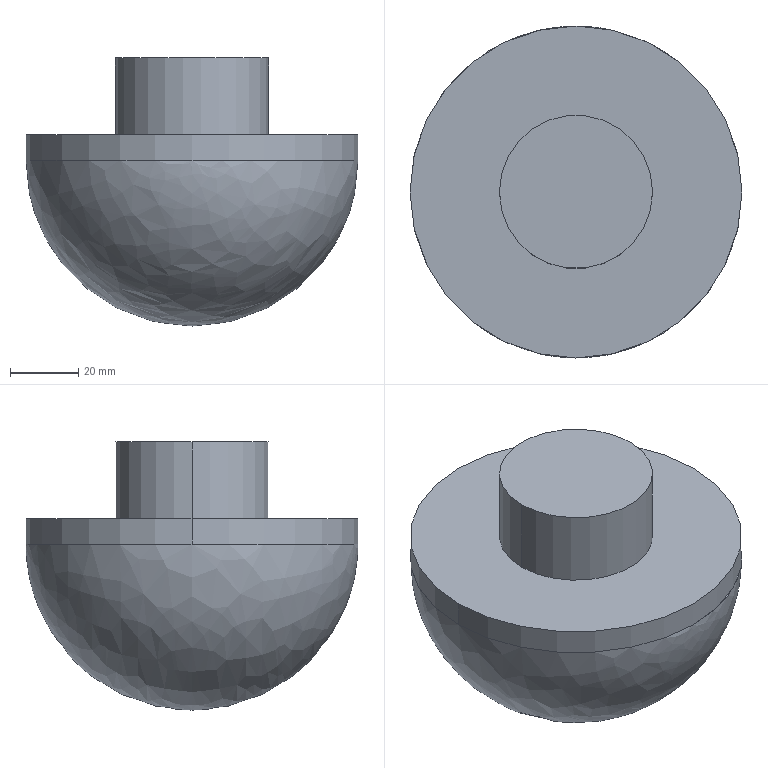Part | SolidWorks | features BaseBody 2, ICE 1, Scale 1 | 2 solids | 10 faces | box 97.5 x 97.5 x 78.75 mm | volume 152963 mm3 | cylinder 4 | plane 4 | spline 2 | commonest cylinder face diameters 45 x2 97.5 x2